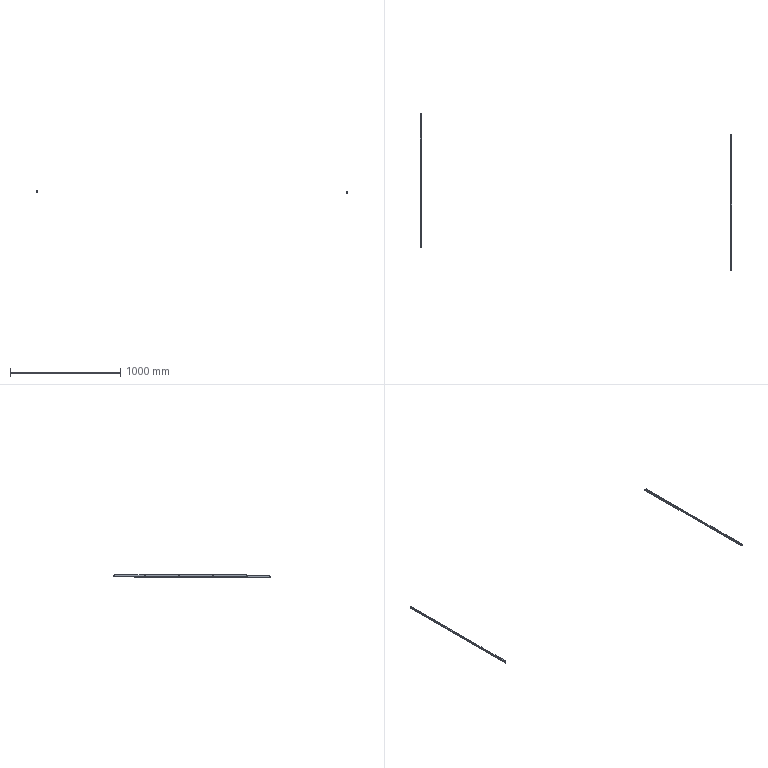Part | 2 solids | 76 faces | box 2829 x 1430 x 20 mm | volume 384714 mm3 | plane 44 | cone 16 | cylinder 16 | commonest cylinder face diameters 3.3 x16